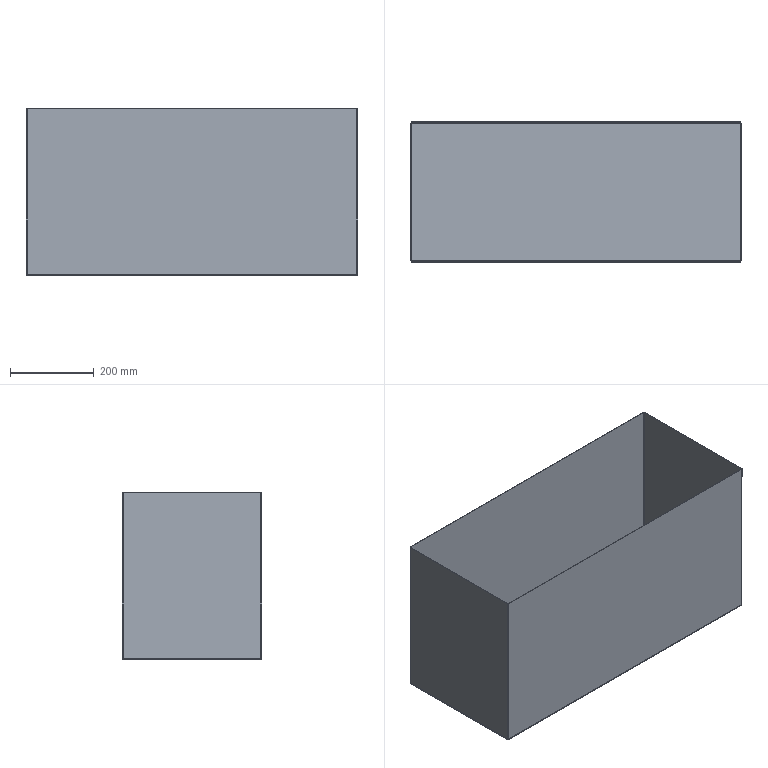Part | SolidWorks | features EdgeFlange 1, FlatPattern 1, SMBaseFlange 1, SheetMetal 1 | 1 solid | 38 faces | box 795 x 335 x 400 mm | volume 2310463 mm3 | plane 22 | spline 8 | cylinder 8 | commonest cylinder face diameters 2 x4 6 x4
STEP:
#1=CARTESIAN_POINT('',(-394.5,-164.5,-2.));
#2=VERTEX_POINT('',#1);
#3=CARTESIAN_POINT('',(-394.5,164.5,-2.));
#4=VERTEX_POINT('',#3);
#5=CARTESIAN_POINT('',(-394.5,-164.793,-2.));
#6=DIRECTION('',(0.,1.,0.));
#7=VECTOR('',#6,1000.);
#8=LINE('',#5,#7);
#9=EDGE_CURVE('',#2,#4,#8,.T.);
#10=ORIENTED_EDGE('',*,*,#9,.T.);
#11=CARTESIAN_POINT('',(394.5,164.5,-2.));
#12=VERTEX_POINT('',#11);
#13=CARTESIAN_POINT('',(-394.793,164.5,-2.));
#14=DIRECTION('',(1.,0.,0.));
#15=VECTOR('',#14,1000.);
#16=LINE('',#13,#15);
#17=EDGE_CURVE('',#4,#12,#16,.T.);
#18=ORIENTED_EDGE('',*,*,#17,.T.);
#19=CARTESIAN_POINT('',(394.5,-164.5,-2.));
#20=VERTEX_POINT('',#19);
#21=CARTESIAN_POINT('',(394.5,164.793,-2.));
#22=DIRECTION('',(0.,-1.,0.));
#23=VECTOR('',#22,1000.);
#24=LINE('',#21,#23);
#25=EDGE_CURVE('',#12,#20,#24,.T.);
#26=ORIENTED_EDGE('',*,*,#25,.T.);
#27=CARTESIAN_POINT('',(394.793,-164.5,-2.));
#28=DIRECTION('',(-1.,0.,0.));
#29=VECTOR('',#28,1000.);
#30=LINE('',#27,#29);
#31=EDGE_CURVE('',#20,#2,#30,.T.);
#32=ORIENTED_EDGE('',*,*,#31,.T.);
#33=EDGE_LOOP('',(#10,#18,#26,#32));
#34=FACE_OUTER_BOUND('',#33,.T.);
#35=CARTESIAN_POINT('',(0.,0.,-2.));
#36=DIRECTION('',(0.,0.,1.));
#37=DIRECTION('',(1.,0.,0.));
#38=AXIS2_PLACEMENT_3D('',#35,#36,#37);
#39=PLANE('',#38);
#40=ADVANCED_FACE('',(#34),#39,.F.);
#41=CARTESIAN_POINT('',(-394.5,164.5,0.));
#42=VERTEX_POINT('',#41);
#43=CARTESIAN_POINT('',(394.5,164.5,0.));
#44=VERTEX_POINT('',#43);
#45=CARTESIAN_POINT('',(-394.793,164.5,0.));
#46=DIRECTION('',(1.,0.,0.));
#47=VECTOR('',#46,1000.);
#48=LINE('',#45,#47);
#49=EDGE_CURVE('',#42,#44,#48,.T.);
#50=ORIENTED_EDGE('',*,*,#49,.F.);
#51=CARTESIAN_POINT('',(-394.5,-164.5,0.));
#52=VERTEX_POINT('',#51);
#53=CARTESIAN_POINT('',(-394.5,-164.793,0.));
#54=DIRECTION('',(0.,1.,0.));
#55=VECTOR('',#54,1000.);
#56=LINE('',#53,#55);
#57=EDGE_CURVE('',#52,#42,#56,.T.);
#58=ORIENTED_EDGE('',*,*,#57,.F.);
#59=CARTESIAN_POINT('',(394.5,-164.5,0.));
#60=VERTEX_POINT('',#59);
#61=CARTESIAN_POINT('',(394.793,-164.5,0.));
#62=DIRECTION('',(-1.,0.,0.));
#63=VECTOR('',#62,1000.);
#64=LINE('',#61,#63);
#65=EDGE_CURVE('',#60,#52,#64,.T.);
#66=ORIENTED_EDGE('',*,*,#65,.F.);
#67=CARTESIAN_POINT('',(394.5,164.793,0.));
#68=DIRECTION('',(0.,-1.,0.));
#69=VECTOR('',#68,1000.);
#70=LINE('',#67,#69);
#71=EDGE_CURVE('',#44,#60,#70,.T.);
#72=ORIENTED_EDGE('',*,*,#71,.F.);
#73=EDGE_LOOP('',(#50,#58,#66,#72));
#74=FACE_OUTER_BOUND('',#73,.T.);
#75=CARTESIAN_POINT('',(0.,0.,0.));
#76=DIRECTION('',(0.,0.,1.));
#77=DIRECTION('',(1.,0.,0.));
#78=AXIS2_PLACEMENT_3D('',#75,#76,#77);
#79=PLANE('',#78);
#80=ADVANCED_FACE('',(#74),#79,.T.);
#81=CARTESIAN_POINT('',(394.793,167.5,1.));
#82=VERTEX_POINT('',#81);
#83=CARTESIAN_POINT('',(394.793,165.5,1.));
#84=VERTEX_POINT('',#83);
#85=CARTESIAN_POINT('',(394.793,165.5,1.));
#86=DIRECTION('',(0.,-1.,0.));
#87=VECTOR('',#86,1000.);
#88=LINE('',#85,#87);
#89=EDGE_CURVE('',#82,#84,#88,.T.);
#90=ORIENTED_EDGE('',*,*,#89,.T.);
#91=CARTESIAN_POINT('',(394.5,164.5,0.));
#92=CARTESIAN_POINT('',(394.549,164.762,0.));
#93=CARTESIAN_POINT('',(394.598,165.022,0.1078));
#94=CARTESIAN_POINT('',(394.695,165.392,0.478));
#95=CARTESIAN_POINT('',(394.744,165.5,0.7382));
#96=CARTESIAN_POINT('',(394.793,165.5,1.));
#97=B_SPLINE_CURVE_WITH_KNOTS('',3,(#91,#92,#93,#94,#95,#96),.UNSPECIFIED.,.F.,.F.,(4,2,4),(0.,0.5,1.),.UNSPECIFIED.);
#98=EDGE_CURVE('',#44,#84,#97,.T.);
#99=ORIENTED_EDGE('',*,*,#98,.F.);
#100=CARTESIAN_POINT('',(394.5,164.5,0.));
#101=DIRECTION('',(0.,0.,-1.));
#102=VECTOR('',#101,1000.);
#103=LINE('',#100,#102);
#104=EDGE_CURVE('',#44,#12,#103,.T.);
#105=ORIENTED_EDGE('',*,*,#104,.T.);
#106=CARTESIAN_POINT('',(394.5,164.5,-2.));
#107=CARTESIAN_POINT('',(394.524,164.893,-2.));
#108=CARTESIAN_POINT('',(394.549,165.285,-1.922));
#109=CARTESIAN_POINT('',(394.598,166.011,-1.621));
#110=CARTESIAN_POINT('',(394.622,166.344,-1.399));
#111=CARTESIAN_POINT('',(394.671,166.899,-0.8436));
#112=CARTESIAN_POINT('',(394.695,167.121,-0.5109));
#113=CARTESIAN_POINT('',(394.744,167.422,0.2148));
#114=CARTESIAN_POINT('',(394.768,167.5,0.6073));
#115=CARTESIAN_POINT('',(394.793,167.5,1.));
#116=B_SPLINE_CURVE_WITH_KNOTS('',3,(#106,#107,#108,#109,#110,#111,#112,#113,#114,#115),.UNSPECIFIED.,.F.,.F.,(4,2,2,2,4),(0.,0.25,0.5,0.75,1.),.UNSPECIFIED.);
#117=EDGE_CURVE('',#12,#82,#116,.T.);
#118=ORIENTED_EDGE('',*,*,#117,.T.);
#119=EDGE_LOOP('',(#90,#99,#105,#118));
#120=FACE_OUTER_BOUND('',#119,.T.);
#121=CARTESIAN_POINT('',(394.5,164.5,-2.02));
#122=CARTESIAN_POINT('',(394.524,164.895,-2.02));
#123=CARTESIAN_POINT('',(394.549,165.29,-1.941));
#124=CARTESIAN_POINT('',(394.598,166.021,-1.639));
#125=CARTESIAN_POINT('',(394.622,166.356,-1.415));
#126=CARTESIAN_POINT('',(394.671,166.915,-0.8559));
#127=CARTESIAN_POINT('',(394.695,167.139,-0.5209));
#128=CARTESIAN_POINT('',(394.744,167.441,0.2095));
#129=CARTESIAN_POINT('',(394.768,167.52,0.6046));
#130=CARTESIAN_POINT('',(394.793,167.52,1.));
#131=CARTESIAN_POINT('',(394.5,164.5,-2.));
#132=CARTESIAN_POINT('',(394.524,164.893,-2.));
#133=CARTESIAN_POINT('',(394.549,165.285,-1.922));
#134=CARTESIAN_POINT('',(394.598,166.011,-1.621));
#135=CARTESIAN_POINT('',(394.622,166.344,-1.399));
#136=CARTESIAN_POINT('',(394.671,166.899,-0.8436));
#137=CARTESIAN_POINT('',(394.695,167.121,-0.5109));
#138=CARTESIAN_POINT('',(394.744,167.422,0.2148));
#139=CARTESIAN_POINT('',(394.768,167.5,0.6072));
#140=CARTESIAN_POINT('',(394.793,167.5,1.));
#141=CARTESIAN_POINT('',(394.5,164.5,0.));
#142=CARTESIAN_POINT('',(394.524,164.631,0.));
#143=CARTESIAN_POINT('',(394.549,164.762,0.02603));
#144=CARTESIAN_POINT('',(394.598,165.004,0.1262));
#145=CARTESIAN_POINT('',(394.622,165.115,0.2003));
#146=CARTESIAN_POINT('',(394.671,165.3,0.3855));
#147=CARTESIAN_POINT('',(394.695,165.374,0.4964));
#148=CARTESIAN_POINT('',(394.744,165.474,0.7383));
#149=CARTESIAN_POINT('',(394.768,165.5,0.8691));
#150=CARTESIAN_POINT('',(394.793,165.5,1.));
#151=CARTESIAN_POINT('',(394.5,164.5,0.0202));
#152=CARTESIAN_POINT('',(394.524,164.628,0.0202));
#153=CARTESIAN_POINT('',(394.549,164.756,0.0457));
#154=CARTESIAN_POINT('',(394.598,164.993,0.1439));
#155=CARTESIAN_POINT('',(394.622,165.102,0.2165));
#156=CARTESIAN_POINT('',(394.671,165.284,0.3979));
#157=CARTESIAN_POINT('',(394.695,165.356,0.5066));
#158=CARTESIAN_POINT('',(394.744,165.454,0.7435));
#159=CARTESIAN_POINT('',(394.768,165.48,0.8717));
#160=CARTESIAN_POINT('',(394.793,165.48,1.));
#161=B_SPLINE_SURFACE_WITH_KNOTS('',1,3,((#121,#122,#123,#124,#125,#126,#127,#128,#129,#130),(#131,#132,#133,#134,#135,#136,#137,#138,#139,#140),(#141,#142,#143,#144,#145,#146,#147,#148,#149,#150),(#151,#152,#153,#154,#155,#156,#157,#158,#159,#160)),.UNSPECIFIED.,.F.,.F.,.F.,(2,1,1,2),(4,2,2,2,4),(-0.01,0.,1.,1.01),(0.,0.25,0.5,0.75,1.),.UNSPECIFIED.);
#162=ADVANCED_FACE('',(#120),#161,.F.);
#163=CARTESIAN_POINT('',(-394.793,165.5,1.));
#164=VERTEX_POINT('',#163);
#165=CARTESIAN_POINT('',(-394.793,165.5,1.));
#166=CARTESIAN_POINT('',(-394.744,165.5,0.7382));
#167=CARTESIAN_POINT('',(-394.695,165.392,0.478));
#168=CARTESIAN_POINT('',(-394.598,165.022,0.1078));
#169=CARTESIAN_POINT('',(-394.549,164.762,0.));
#170=CARTESIAN_POINT('',(-394.5,164.5,0.));
#171=B_SPLINE_CURVE_WITH_KNOTS('',3,(#165,#166,#167,#168,#169,#170),.UNSPECIFIED.,.F.,.F.,(4,2,4),(0.,0.5,1.),.UNSPECIFIED.);
#172=EDGE_CURVE('',#164,#42,#171,.T.);
#173=ORIENTED_EDGE('',*,*,#172,.F.);
#174=CARTESIAN_POINT('',(-394.793,167.5,1.));
#175=VERTEX_POINT('',#174);
#176=CARTESIAN_POINT('',(-394.793,165.5,1.));
#177=DIRECTION('',(0.,-1.,0.));
#178=VECTOR('',#177,1000.);
#179=LINE('',#176,#178);
#180=EDGE_CURVE('',#175,#164,#179,.T.);
#181=ORIENTED_EDGE('',*,*,#180,.F.);
#182=CARTESIAN_POINT('',(-394.793,167.5,1.));
#183=CARTESIAN_POINT('',(-394.768,167.5,0.6073));
#184=CARTESIAN_POINT('',(-394.744,167.422,0.2148));
#185=CARTESIAN_POINT('',(-394.695,167.121,-0.5109));
#186=CARTESIAN_POINT('',(-394.671,166.899,-0.8436));
#187=CARTESIAN_POINT('',(-394.622,166.344,-1.399));
#188=CARTESIAN_POINT('',(-394.598,166.011,-1.621));
#189=CARTESIAN_POINT('',(-394.549,165.285,-1.922));
#190=CARTESIAN_POINT('',(-394.524,164.893,-2.));
#191=CARTESIAN_POINT('',(-394.5,164.5,-2.));
#192=B_SPLINE_CURVE_WITH_KNOTS('',3,(#182,#183,#184,#185,#186,#187,#188,#189,#190,#191),.UNSPECIFIED.,.F.,.F.,(4,2,2,2,4),(0.,0.25,0.5,0.75,1.),.UNSPECIFIED.);
#193=EDGE_CURVE('',#175,#4,#192,.T.);
#194=ORIENTED_EDGE('',*,*,#193,.T.);
#195=CARTESIAN_POINT('',(-394.5,164.5,0.));
#196=DIRECTION('',(0.,0.,-1.));
#197=VECTOR('',#196,1000.);
#198=LINE('',#195,#197);
#199=EDGE_CURVE('',#42,#4,#198,.T.);
#200=ORIENTED_EDGE('',*,*,#199,.F.);
#201=EDGE_LOOP('',(#173,#181,#194,#200));
#202=FACE_OUTER_BOUND('',#201,.T.);
#203=CARTESIAN_POINT('',(-394.793,167.52,1.));
#204=CARTESIAN_POINT('',(-394.768,167.52,0.6046));
#205=CARTESIAN_POINT('',(-394.744,167.441,0.2095));
#206=CARTESIAN_POINT('',(-394.695,167.139,-0.5209));
#207=CARTESIAN_POINT('',(-394.671,166.915,-0.8559));
#208=CARTESIAN_POINT('',(-394.622,166.356,-1.415));
#209=CARTESIAN_POINT('',(-394.598,166.021,-1.639));
#210=CARTESIAN_POINT('',(-394.549,165.29,-1.941));
#211=CARTESIAN_POINT('',(-394.524,164.895,-2.02));
#212=CARTESIAN_POINT('',(-394.5,164.5,-2.02));
#213=CARTESIAN_POINT('',(-394.793,167.5,1.));
#214=CARTESIAN_POINT('',(-394.768,167.5,0.6072));
#215=CARTESIAN_POINT('',(-394.744,167.422,0.2148));
#216=CARTESIAN_POINT('',(-394.695,167.121,-0.5109));
#217=CARTESIAN_POINT('',(-394.671,166.899,-0.8436));
#218=CARTESIAN_POINT('',(-394.622,166.344,-1.399));
#219=CARTESIAN_POINT('',(-394.598,166.011,-1.621));
#220=CARTESIAN_POINT('',(-394.549,165.285,-1.922));
#221=CARTESIAN_POINT('',(-394.524,164.893,-2.));
#222=CARTESIAN_POINT('',(-394.5,164.5,-2.));
#223=CARTESIAN_POINT('',(-394.793,165.5,1.));
#224=CARTESIAN_POINT('',(-394.768,165.5,0.8691));
#225=CARTESIAN_POINT('',(-394.744,165.474,0.7383));
#226=CARTESIAN_POINT('',(-394.695,165.374,0.4964));
#227=CARTESIAN_POINT('',(-394.671,165.3,0.3855));
#228=CARTESIAN_POINT('',(-394.622,165.115,0.2003));
#229=CARTESIAN_POINT('',(-394.598,165.004,0.1262));
#230=CARTESIAN_POINT('',(-394.549,164.762,0.02603));
#231=CARTESIAN_POINT('',(-394.524,164.631,0.));
#232=CARTESIAN_POINT('',(-394.5,164.5,0.));
#233=CARTESIAN_POINT('',(-394.793,165.48,1.));
#234=CARTESIAN_POINT('',(-394.768,165.48,0.8717));
#235=CARTESIAN_POINT('',(-394.744,165.454,0.7435));
#236=CARTESIAN_POINT('',(-394.695,165.356,0.5066));
#237=CARTESIAN_POINT('',(-394.671,165.284,0.3979));
#238=CARTESIAN_POINT('',(-394.622,165.102,0.2165));
#239=CARTESIAN_POINT('',(-394.598,164.993,0.1439));
#240=CARTESIAN_POINT('',(-394.549,164.756,0.0457));
#241=CARTESIAN_POINT('',(-394.524,164.628,0.0202));
#242=CARTESIAN_POINT('',(-394.5,164.5,0.0202));
#243=B_SPLINE_SURFACE_WITH_KNOTS('',1,3,((#203,#204,#205,#206,#207,#208,#209,#210,#211,#212),(#213,#214,#215,#216,#217,#218,#219,#220,#221,#222),(#223,#224,#225,#226,#227,#228,#229,#230,#231,#232),(#233,#234,#235,#236,#237,#238,#239,#240,#241,#242)),.UNSPECIFIED.,.F.,.F.,.F.,(2,1,1,2),(4,2,2,2,4),(-0.01,0.,1.,1.01),(0.,0.25,0.5,0.75,1.),.UNSPECIFIED.);
#244=ADVANCED_FACE('',(#202),#243,.F.);
#245=ORIENTED_EDGE('',*,*,#17,.F.);
#246=ORIENTED_EDGE('',*,*,#193,.F.);
#247=CARTESIAN_POINT('',(397.5,167.5,1.));
#248=DIRECTION('',(1.,0.,0.));
#249=VECTOR('',#248,1000.);
#250=LINE('',#247,#249);
#251=EDGE_CURVE('',#175,#82,#250,.T.);
#252=ORIENTED_EDGE('',*,*,#251,.T.);
#253=ORIENTED_EDGE('',*,*,#117,.F.);
#254=EDGE_LOOP('',(#245,#246,#252,#253));
#255=FACE_OUTER_BOUND('',#254,.T.);
#256=CARTESIAN_POINT('',(-394.793,164.5,1.));
#257=DIRECTION('',(-1.,0.,0.));
#258=DIRECTION('',(0.,1.,0.));
#259=AXIS2_PLACEMENT_3D('',#256,#257,#258);
#260=CYLINDRICAL_SURFACE('',#259,3.);
#261=ADVANCED_FACE('',(#255),#260,.T.);
#262=ORIENTED_EDGE('',*,*,#49,.T.);
#263=ORIENTED_EDGE('',*,*,#98,.T.);
#264=CARTESIAN_POINT('',(397.5,165.5,1.));
#265=DIRECTION('',(-1.,0.,0.));
#266=VECTOR('',#265,1000.);
#267=LINE('',#264,#266);
#268=EDGE_CURVE('',#84,#164,#267,.T.);
#269=ORIENTED_EDGE('',*,*,#268,.T.);
#270=ORIENTED_EDGE('',*,*,#172,.T.);
#271=EDGE_LOOP('',(#262,#263,#269,#270));
#272=FACE_OUTER_BOUND('',#271,.T.);
#273=CARTESIAN_POINT('',(-394.793,164.5,1.));
#274=DIRECTION('',(-1.,0.,0.));
#275=DIRECTION('',(0.,1.,0.));
#276=AXIS2_PLACEMENT_3D('',#273,#274,#275);
#277=CYLINDRICAL_SURFACE('',#276,1.);
#278=ADVANCED_FACE('',(#272),#277,.F.);
#279=CARTESIAN_POINT('',(394.793,167.5,398.));
#280=VERTEX_POINT('',#279);
#281=CARTESIAN_POINT('',(394.793,167.5,0.));
#282=DIRECTION('',(0.,0.,1.));
#283=VECTOR('',#282,1000.);
#284=LINE('',#281,#283);
#285=EDGE_CURVE('',#82,#280,#284,.T.);
#286=ORIENTED_EDGE('',*,*,#285,.T.);
#287=CARTESIAN_POINT('',(394.793,165.5,398.));
#288=VERTEX_POINT('',#287);
#289=CARTESIAN_POINT('',(394.793,165.5,398.));
#290=DIRECTION('',(0.,-1.,0.));
#291=VECTOR('',#290,1000.);
#292=LINE('',#289,#291);
#293=EDGE_CURVE('',#280,#288,#292,.T.);
#294=ORIENTED_EDGE('',*,*,#293,.T.);
#295=CARTESIAN_POINT('',(394.793,165.5,0.));
#296=DIRECTION('',(0.,0.,1.));
#297=VECTOR('',#296,1000.);
#298=LINE('',#295,#297);
#299=EDGE_CURVE('',#84,#288,#298,.T.);
#300=ORIENTED_EDGE('',*,*,#299,.F.);
#301=ORIENTED_EDGE('',*,*,#89,.F.);
#302=EDGE_LOOP('',(#286,#294,#300,#301));
#303=FACE_OUTER_BOUND('',#302,.T.);
#304=CARTESIAN_POINT('',(394.793,165.5,0.));
#305=DIRECTION('',(1.,0.,0.));
#306=DIRECTION('',(0.,0.,-1.));
#307=AXIS2_PLACEMENT_3D('',#304,#305,#306);
#308=PLANE('',#307);
#309=ADVANCED_FACE('',(#303),#308,.T.);
#310=ORIENTED_EDGE('',*,*,#251,.F.);
#311=CARTESIAN_POINT('',(-394.793,167.5,398.));
#312=VERTEX_POINT('',#311);
#313=CARTESIAN_POINT('',(-394.793,167.5,0.));
#314=DIRECTION('',(0.,0.,1.));
#315=VECTOR('',#314,1000.);
#316=LINE('',#313,#315);
#317=EDGE_CURVE('',#175,#312,#316,.T.);
#318=ORIENTED_EDGE('',*,*,#317,.T.);
#319=CARTESIAN_POINT('',(0.,167.5,398.));
#320=DIRECTION('',(1.,0.,0.));
#321=VECTOR('',#320,1000.);
#322=LINE('',#319,#321);
#323=EDGE_CURVE('',#312,#280,#322,.T.);
#324=ORIENTED_EDGE('',*,*,#323,.T.);
#325=ORIENTED_EDGE('',*,*,#285,.F.);
#326=EDGE_LOOP('',(#310,#318,#324,#325));
#327=FACE_OUTER_BOUND('',#326,.T.);
#328=CARTESIAN_POINT('',(0.,167.5,0.));
#329=DIRECTION('',(0.,-1.,0.));
#330=DIRECTION('',(0.,0.,-1.));
#331=AXIS2_PLACEMENT_3D('',#328,#329,#330);
#332=PLANE('',#331);
#333=ADVANCED_FACE('',(#327),#332,.F.);
#334=CARTESIAN_POINT('',(-394.793,165.5,398.));
#335=VERTEX_POINT('',#334);
#336=CARTESIAN_POINT('',(-394.793,165.5,0.));
#337=DIRECTION('',(0.,0.,1.));
#338=VECTOR('',#337,1000.);
#339=LINE('',#336,#338);
#340=EDGE_CURVE('',#164,#335,#339,.T.);
#341=ORIENTED_EDGE('',*,*,#340,.F.);
#342=ORIENTED_EDGE('',*,*,#268,.F.);
#343=ORIENTED_EDGE('',*,*,#299,.T.);
#344=CARTESIAN_POINT('',(397.5,165.5,398.));
#345=DIRECTION('',(1.,0.,0.));
#346=VECTOR('',#345,1000.);
#347=LINE('',#344,#346);
#348=EDGE_CURVE('',#335,#288,#347,.T.);
#349=ORIENTED_EDGE('',*,*,#348,.F.);
#350=EDGE_LOOP('',(#341,#342,#343,#349));
#351=FACE_OUTER_BOUND('',#350,.T.);
#352=CARTESIAN_POINT('',(0.,165.5,0.));
#353=DIRECTION('',(0.,-1.,0.));
#354=DIRECTION('',(0.,0.,-1.));
#355=AXIS2_PLACEMENT_3D('',#352,#353,#354);
#356=PLANE('',#355);
#357=ADVANCED_FACE('',(#351),#356,.T.);
#358=ORIENTED_EDGE('',*,*,#323,.F.);
#359=CARTESIAN_POINT('',(-394.793,167.5,398.));
#360=DIRECTION('',(0.,-1.,0.));
#361=VECTOR('',#360,1000.);
#362=LINE('',#359,#361);
#363=EDGE_CURVE('',#312,#335,#362,.T.);
#364=ORIENTED_EDGE('',*,*,#363,.T.);
#365=ORIENTED_EDGE('',*,*,#348,.T.);
#366=ORIENTED_EDGE('',*,*,#293,.F.);
#367=EDGE_LOOP('',(#358,#364,#365,#366));
#368=FACE_OUTER_BOUND('',#367,.T.);
#369=CARTESIAN_POINT('',(397.5,167.5,398.));
#370=DIRECTION('',(0.,0.,-1.));
#371=DIRECTION('',(0.,1.,0.));
#372=AXIS2_PLACEMENT_3D('',#369,#370,#371);
#373=PLANE('',#372);
#374=ADVANCED_FACE('',(#368),#373,.F.);
#375=ORIENTED_EDGE('',*,*,#363,.F.);
#376=ORIENTED_EDGE('',*,*,#317,.F.);
#377=ORIENTED_EDGE('',*,*,#180,.T.);
#378=ORIENTED_EDGE('',*,*,#340,.T.);
#379=EDGE_LOOP('',(#375,#376,#377,#378));
#380=FACE_OUTER_BOUND('',#379,.T.);
#381=CARTESIAN_POINT('',(-394.793,165.5,0.));
#382=DIRECTION('',(1.,0.,0.));
#383=DIRECTION('',(0.,0.,-1.));
#384=AXIS2_PLACEMENT_3D('',#381,#382,#383);
#385=PLANE('',#384);
#386=ADVANCED_FACE('',(#380),#385,.F.);
#387=CARTESIAN_POINT('',(-394.793,-167.5,1.));
#388=VERTEX_POINT('',#387);
#389=CARTESIAN_POINT('',(-394.793,-165.5,1.));
#390=VERTEX_POINT('',#389);
#391=CARTESIAN_POINT('',(-394.793,-165.5,1.));
#392=DIRECTION('',(0.,1.,0.));
#393=VECTOR('',#392,1000.);
#394=LINE('',#391,#393);
#395=EDGE_CURVE('',#388,#390,#394,.T.);
#396=ORIENTED_EDGE('',*,*,#395,.T.);
#397=CARTESIAN_POINT('',(-394.5,-164.5,0.));
#398=CARTESIAN_POINT('',(-394.549,-164.762,0.));
#399=CARTESIAN_POINT('',(-394.598,-165.022,0.1078));
#400=CARTESIAN_POINT('',(-394.695,-165.392,0.478));
#401=CARTESIAN_POINT('',(-394.744,-165.5,0.7382));
#402=CARTESIAN_POINT('',(-394.793,-165.5,1.));
#403=B_SPLINE_CURVE_WITH_KNOTS('',3,(#397,#398,#399,#400,#401,#402),.UNSPECIFIED.,.F.,.F.,(4,2,4),(0.,0.5,1.),.UNSPECIFIED.);
#404=EDGE_CURVE('',#52,#390,#403,.T.);
#405=ORIENTED_EDGE('',*,*,#404,.F.);
#406=CARTESIAN_POINT('',(-394.5,-164.5,0.));
#407=DIRECTION('',(0.,0.,-1.));
#408=VECTOR('',#407,1000.);
#409=LINE('',#406,#408);
#410=EDGE_CURVE('',#52,#2,#409,.T.);
#411=ORIENTED_EDGE('',*,*,#410,.T.);
#412=CARTESIAN_POINT('',(-394.5,-164.5,-2.));
#413=CARTESIAN_POINT('',(-394.524,-164.893,-2.));
#414=CARTESIAN_POINT('',(-394.549,-165.285,-1.922));
#415=CARTESIAN_POINT('',(-394.598,-166.011,-1.621));
#416=CARTESIAN_POINT('',(-394.622,-166.344,-1.399));
#417=CARTESIAN_POINT('',(-394.671,-166.899,-0.8436));
#418=CARTESIAN_POINT('',(-394.695,-167.121,-0.5109));
#419=CARTESIAN_POINT('',(-394.744,-167.422,0.2148));
#420=CARTESIAN_POINT('',(-394.768,-167.5,0.6073));
#421=CARTESIAN_POINT('',(-394.793,-167.5,1.));
#422=B_SPLINE_CURVE_WITH_KNOTS('',3,(#412,#413,#414,#415,#416,#417,#418,#419,#420,#421),.UNSPECIFIED.,.F.,.F.,(4,2,2,2,4),(0.,0.25,0.5,0.75,1.),.UNSPECIFIED.);
#423=EDGE_CURVE('',#2,#388,#422,.T.);
#424=ORIENTED_EDGE('',*,*,#423,.T.);
#425=EDGE_LOOP('',(#396,#405,#411,#424));
#426=FACE_OUTER_BOUND('',#425,.T.);
#427=CARTESIAN_POINT('',(-394.5,-164.5,-2.02));
#428=CARTESIAN_POINT('',(-394.524,-164.895,-2.02));
#429=CARTESIAN_POINT('',(-394.549,-165.29,-1.941));
#430=CARTESIAN_POINT('',(-394.598,-166.021,-1.639));
#431=CARTESIAN_POINT('',(-394.622,-166.356,-1.415));
#432=CARTESIAN_POINT('',(-394.671,-166.915,-0.8559));
#433=CARTESIAN_POINT('',(-394.695,-167.139,-0.5209));
#434=CARTESIAN_POINT('',(-394.744,-167.441,0.2095));
#435=CARTESIAN_POINT('',(-394.768,-167.52,0.6046));
#436=CARTESIAN_POINT('',(-394.793,-167.52,1.));
#437=CARTESIAN_POINT('',(-394.5,-164.5,-2.));
#438=CARTESIAN_POINT('',(-394.524,-164.893,-2.));
#439=CARTESIAN_POINT('',(-394.549,-165.285,-1.922));
#440=CARTESIAN_POINT('',(-394.598,-166.011,-1.621));
#441=CARTESIAN_POINT('',(-394.622,-166.344,-1.399));
#442=CARTESIAN_POINT('',(-394.671,-166.899,-0.8436));
#443=CARTESIAN_POINT('',(-394.695,-167.121,-0.5109));
#444=CARTESIAN_POINT('',(-394.744,-167.422,0.2148));
#445=CARTESIAN_POINT('',(-394.768,-167.5,0.6072));
#446=CARTESIAN_POINT('',(-394.793,-167.5,1.));
#447=CARTESIAN_POINT('',(-394.5,-164.5,0.));
#448=CARTESIAN_POINT('',(-394.524,-164.631,0.));
#449=CARTESIAN_POINT('',(-394.549,-164.762,0.02603));
#450=CARTESIAN_POINT('',(-394.598,-165.004,0.1262));
#451=CARTESIAN_POINT('',(-394.622,-165.115,0.2003));
#452=CARTESIAN_POINT('',(-394.671,-165.3,0.3855));
#453=CARTESIAN_POINT('',(-394.695,-165.374,0.4964));
#454=CARTESIAN_POINT('',(-394.744,-165.474,0.7383));
#455=CARTESIAN_POINT('',(-394.768,-165.5,0.8691));
#456=CARTESIAN_POINT('',(-394.793,-165.5,1.));
#457=CARTESIAN_POINT('',(-394.5,-164.5,0.0202));
#458=CARTESIAN_POINT('',(-394.524,-164.628,0.0202));
#459=CARTESIAN_POINT('',(-394.549,-164.756,0.0457));
#460=CARTESIAN_POINT('',(-394.598,-164.993,0.1439));
#461=CARTESIAN_POINT('',(-394.622,-165.102,0.2165));
#462=CARTESIAN_POINT('',(-394.671,-165.284,0.3979));
#463=CARTESIAN_POINT('',(-394.695,-165.356,0.5066));
#464=CARTESIAN_POINT('',(-394.744,-165.454,0.7435));
#465=CARTESIAN_POINT('',(-394.768,-165.48,0.8717));
#466=CARTESIAN_POINT('',(-394.793,-165.48,1.));
#467=B_SPLINE_SURFACE_WITH_KNOTS('',1,3,((#427,#428,#429,#430,#431,#432,#433,#434,#435,#436),(#437,#438,#439,#440,#441,#442,#443,#444,#445,#446),(#447,#448,#449,#450,#451,#452,#453,#454,#455,#456),(#457,#458,#459,#460,#461,#462,#463,#464,#465,#466)),.UNSPECIFIED.,.F.,.F.,.F.,(2,1,1,2),(4,2,2,2,4),(-0.01,0.,1.,1.01),(0.,0.25,0.5,0.75,1.),.UNSPECIFIED.);
#468=ADVANCED_FACE('',(#426),#467,.F.);
#469=CARTESIAN_POINT('',(394.793,-165.5,1.));
#470=VERTEX_POINT('',#469);
#471=CARTESIAN_POINT('',(394.793,-165.5,1.));
#472=CARTESIAN_POINT('',(394.744,-165.5,0.7382));
#473=CARTESIAN_POINT('',(394.695,-165.392,0.478));
#474=CARTESIAN_POINT('',(394.598,-165.022,0.1078));
#475=CARTESIAN_POINT('',(394.549,-164.762,0.));
#476=CARTESIAN_POINT('',(394.5,-164.5,0.));
#477=B_SPLINE_CURVE_WITH_KNOTS('',3,(#471,#472,#473,#474,#475,#476),.UNSPECIFIED.,.F.,.F.,(4,2,4),(0.,0.5,1.),.UNSPECIFIED.);
#478=EDGE_CURVE('',#470,#60,#477,.T.);
#479=ORIENTED_EDGE('',*,*,#478,.F.);
#480=CARTESIAN_POINT('',(394.793,-167.5,1.));
#481=VERTEX_POINT('',#480);
#482=CARTESIAN_POINT('',(394.793,-165.5,1.));
#483=DIRECTION('',(0.,1.,0.));
#484=VECTOR('',#483,1000.);
#485=LINE('',#482,#484);
#486=EDGE_CURVE('',#481,#470,#485,.T.);
#487=ORIENTED_EDGE('',*,*,#486,.F.);
#488=CARTESIAN_POINT('',(394.793,-167.5,1.));
#489=CARTESIAN_POINT('',(394.768,-167.5,0.6073));
#490=CARTESIAN_POINT('',(394.744,-167.422,0.2148));
#491=CARTESIAN_POINT('',(394.695,-167.121,-0.5109));
#492=CARTESIAN_POINT('',(394.671,-166.899,-0.8436));
#493=CARTESIAN_POINT('',(394.622,-166.344,-1.399));
#494=CARTESIAN_POINT('',(394.598,-166.011,-1.621));
#495=CARTESIAN_POINT('',(394.549,-165.285,-1.922));
#496=CARTESIAN_POINT('',(394.524,-164.893,-2.));
#497=CARTESIAN_POINT('',(394.5,-164.5,-2.));
#498=B_SPLINE_CURVE_WITH_KNOTS('',3,(#488,#489,#490,#491,#492,#493,#494,#495,#496,#497),.UNSPECIFIED.,.F.,.F.,(4,2,2,2,4),(0.,0.25,0.5,0.75,1.),.UNSPECIFIED.);
#499=EDGE_CURVE('',#481,#20,#498,.T.);
#500=ORIENTED_EDGE('',*,*,#499,.T.);
#501=CARTESIAN_POINT('',(394.5,-164.5,0.));
#502=DIRECTION('',(0.,0.,-1.));
#503=VECTOR('',#502,1000.);
#504=LINE('',#501,#503);
#505=EDGE_CURVE('',#60,#20,#504,.T.);
#506=ORIENTED_EDGE('',*,*,#505,.F.);
#507=EDGE_LOOP('',(#479,#487,#500,#506));
#508=FACE_OUTER_BOUND('',#507,.T.);
#509=CARTESIAN_POINT('',(394.793,-167.52,1.));
#510=CARTESIAN_POINT('',(394.768,-167.52,0.6046));
#511=CARTESIAN_POINT('',(394.744,-167.441,0.2095));
#512=CARTESIAN_POINT('',(394.695,-167.139,-0.5209));
#513=CARTESIAN_POINT('',(394.671,-166.915,-0.8559));
#514=CARTESIAN_POINT('',(394.622,-166.356,-1.415));
#515=CARTESIAN_POINT('',(394.598,-166.021,-1.639));
#516=CARTESIAN_POINT('',(394.549,-165.29,-1.941));
#517=CARTESIAN_POINT('',(394.524,-164.895,-2.02));
#518=CARTESIAN_POINT('',(394.5,-164.5,-2.02));
#519=CARTESIAN_POINT('',(394.793,-167.5,1.));
#520=CARTESIAN_POINT('',(394.768,-167.5,0.6072));
#521=CARTESIAN_POINT('',(394.744,-167.422,0.2148));
#522=CARTESIAN_POINT('',(394.695,-167.121,-0.5109));
#523=CARTESIAN_POINT('',(394.671,-166.899,-0.8436));
#524=CARTESIAN_POINT('',(394.622,-166.344,-1.399));
#525=CARTESIAN_POINT('',(394.598,-166.011,-1.621));
#526=CARTESIAN_POINT('',(394.549,-165.285,-1.922));
#527=CARTESIAN_POINT('',(394.524,-164.893,-2.));
#528=CARTESIAN_POINT('',(394.5,-164.5,-2.));
#529=CARTESIAN_POINT('',(394.793,-165.5,1.));
#530=CARTESIAN_POINT('',(394.768,-165.5,0.8691));
#531=CARTESIAN_POINT('',(394.744,-165.474,0.7383));
#532=CARTESIAN_POINT('',(394.695,-165.374,0.4964));
#533=CARTESIAN_POINT('',(394.671,-165.3,0.3855));
#534=CARTESIAN_POINT('',(394.622,-165.115,0.2003));
#535=CARTESIAN_POINT('',(394.598,-165.004,0.1262));
#536=CARTESIAN_POINT('',(394.549,-164.762,0.02603));
#537=CARTESIAN_POINT('',(394.524,-164.631,0.));
#538=CARTESIAN_POINT('',(394.5,-164.5,0.));
#539=CARTESIAN_POINT('',(394.793,-165.48,1.));
#540=CARTESIAN_POINT('',(394.768,-165.48,0.8717));
#541=CARTESIAN_POINT('',(394.744,-165.454,0.7435));
#542=CARTESIAN_POINT('',(394.695,-165.356,0.5066));
#543=CARTESIAN_POINT('',(394.671,-165.284,0.3979));
#544=CARTESIAN_POINT('',(394.622,-165.102,0.2165));
#545=CARTESIAN_POINT('',(394.598,-164.993,0.1439));
#546=CARTESIAN_POINT('',(394.549,-164.756,0.0457));
#547=CARTESIAN_POINT('',(394.524,-164.628,0.0202));
#548=CARTESIAN_POINT('',(394.5,-164.5,0.0202));
#549=B_SPLINE_SURFACE_WITH_KNOTS('',1,3,((#509,#510,#511,#512,#513,#514,#515,#516,#517,#518),(#519,#520,#521,#522,#523,#524,#525,#526,#527,#528),(#529,#530,#531,#532,#533,#534,#535,#536,#537,#538),(#539,#540,#541,#542,#543,#544,#545,#546,#547,#548)),.UNSPECIFIED.,.F.,.F.,.F.,(2,1,1,2),(4,2,2,2,4),(-0.01,0.,1.,1.01),(0.,0.25,0.5,0.75,1.),.UNSPECIFIED.);
#550=ADVANCED_FACE('',(#508),#549,.F.);
#551=ORIENTED_EDGE('',*,*,#31,.F.);
#552=ORIENTED_EDGE('',*,*,#499,.F.);
#553=CARTESIAN_POINT('',(-397.5,-167.5,1.));
#554=DIRECTION('',(-1.,0.,0.));
#555=VECTOR('',#554,1000.);
#556=LINE('',#553,#555);
#557=EDGE_CURVE('',#481,#388,#556,.T.);
#558=ORIENTED_EDGE('',*,*,#557,.T.);
#559=ORIENTED_EDGE('',*,*,#423,.F.);
#560=EDGE_LOOP('',(#551,#552,#558,#559));
#561=FACE_OUTER_BOUND('',#560,.T.);
#562=CARTESIAN_POINT('',(394.793,-164.5,1.));
#563=DIRECTION('',(1.,0.,0.));
#564=DIRECTION('',(0.,-1.,0.));
#565=AXIS2_PLACEMENT_3D('',#562,#563,#564);
#566=CYLINDRICAL_SURFACE('',#565,3.);
#567=ADVANCED_FACE('',(#561),#566,.T.);
#568=ORIENTED_EDGE('',*,*,#65,.T.);
#569=ORIENTED_EDGE('',*,*,#404,.T.);
#570=CARTESIAN_POINT('',(-397.5,-165.5,1.));
#571=DIRECTION('',(1.,0.,0.));
#572=VECTOR('',#571,1000.);
#573=LINE('',#570,#572);
#574=EDGE_CURVE('',#390,#470,#573,.T.);
#575=ORIENTED_EDGE('',*,*,#574,.T.);
#576=ORIENTED_EDGE('',*,*,#478,.T.);
#577=EDGE_LOOP('',(#568,#569,#575,#576));
#578=FACE_OUTER_BOUND('',#577,.T.);
#579=CARTESIAN_POINT('',(394.793,-164.5,1.));
#580=DIRECTION('',(1.,0.,0.));
#581=DIRECTION('',(0.,-1.,0.));
#582=AXIS2_PLACEMENT_3D('',#579,#580,#581);
#583=CYLINDRICAL_SURFACE('',#582,1.);
#584=ADVANCED_FACE('',(#578),#583,.F.);
#585=CARTESIAN_POINT('',(-394.793,-167.5,398.));
#586=VERTEX_POINT('',#585);
#587=CARTESIAN_POINT('',(-394.793,-167.5,0.));
#588=DIRECTION('',(0.,0.,1.));
#589=VECTOR('',#588,1000.);
#590=LINE('',#587,#589);
#591=EDGE_CURVE('',#388,#586,#590,.T.);
#592=ORIENTED_EDGE('',*,*,#591,.T.);
#593=CARTESIAN_POINT('',(-394.793,-165.5,398.));
#594=VERTEX_POINT('',#593);
#595=CARTESIAN_POINT('',(-394.793,-165.5,398.));
#596=DIRECTION('',(0.,1.,0.));
#597=VECTOR('',#596,1000.);
#598=LINE('',#595,#597);
#599=EDGE_CURVE('',#586,#594,#598,.T.);
#600=ORIENTED_EDGE('',*,*,#599,.T.);
#601=CARTESIAN_POINT('',(-394.793,-165.5,0.));
#602=DIRECTION('',(0.,0.,1.));
#603=VECTOR('',#602,1000.);
#604=LINE('',#601,#603);
#605=EDGE_CURVE('',#390,#594,#604,.T.);
#606=ORIENTED_EDGE('',*,*,#605,.F.);
#607=ORIENTED_EDGE('',*,*,#395,.F.);
#608=EDGE_LOOP('',(#592,#600,#606,#607));
#609=FACE_OUTER_BOUND('',#608,.T.);
#610=CARTESIAN_POINT('',(-394.793,-165.5,0.));
#611=DIRECTION('',(-1.,0.,0.));
#612=DIRECTION('',(0.,0.,1.));
#613=AXIS2_PLACEMENT_3D('',#610,#611,#612);
#614=PLANE('',#613);
#615=ADVANCED_FACE('',(#609),#614,.T.);
#616=ORIENTED_EDGE('',*,*,#557,.F.);
#617=CARTESIAN_POINT('',(394.793,-167.5,398.));
#618=VERTEX_POINT('',#617);
#619=CARTESIAN_POINT('',(394.793,-167.5,0.));
#620=DIRECTION('',(0.,0.,1.));
#621=VECTOR('',#620,1000.);
#622=LINE('',#619,#621);
#623=EDGE_CURVE('',#481,#618,#622,.T.);
#624=ORIENTED_EDGE('',*,*,#623,.T.);
#625=CARTESIAN_POINT('',(0.,-167.5,398.));
#626=DIRECTION('',(-1.,0.,0.));
#627=VECTOR('',#626,1000.);
#628=LINE('',#625,#627);
#629=EDGE_CURVE('',#618,#586,#628,.T.);
#630=ORIENTED_EDGE('',*,*,#629,.T.);
#631=ORIENTED_EDGE('',*,*,#591,.F.);
#632=EDGE_LOOP('',(#616,#624,#630,#631));
#633=FACE_OUTER_BOUND('',#632,.T.);
#634=CARTESIAN_POINT('',(0.,-167.5,0.));
#635=DIRECTION('',(0.,1.,0.));
#636=DIRECTION('',(0.,0.,1.));
#637=AXIS2_PLACEMENT_3D('',#634,#635,#636);
#638=PLANE('',#637);
#639=ADVANCED_FACE('',(#633),#638,.F.);
#640=CARTESIAN_POINT('',(394.793,-165.5,398.));
#641=VERTEX_POINT('',#640);
#642=CARTESIAN_POINT('',(394.793,-165.5,0.));
#643=DIRECTION('',(0.,0.,1.));
#644=VECTOR('',#643,1000.);
#645=LINE('',#642,#644);
#646=EDGE_CURVE('',#470,#641,#645,.T.);
#647=ORIENTED_EDGE('',*,*,#646,.F.);
#648=ORIENTED_EDGE('',*,*,#574,.F.);
#649=ORIENTED_EDGE('',*,*,#605,.T.);
#650=CARTESIAN_POINT('',(-397.5,-165.5,398.));
#651=DIRECTION('',(-1.,0.,0.));
#652=VECTOR('',#651,1000.);
#653=LINE('',#650,#652);
#654=EDGE_CURVE('',#641,#594,#653,.T.);
#655=ORIENTED_EDGE('',*,*,#654,.F.);
#656=EDGE_LOOP('',(#647,#648,#649,#655));
#657=FACE_OUTER_BOUND('',#656,.T.);
#658=CARTESIAN_POINT('',(0.,-165.5,0.));
#659=DIRECTION('',(0.,1.,0.));
#660=DIRECTION('',(0.,0.,1.));
#661=AXIS2_PLACEMENT_3D('',#658,#659,#660);
#662=PLANE('',#661);
#663=ADVANCED_FACE('',(#657),#662,.T.);
#664=ORIENTED_EDGE('',*,*,#629,.F.);
#665=CARTESIAN_POINT('',(394.793,-167.5,398.));
#666=DIRECTION('',(0.,1.,0.));
#667=VECTOR('',#666,1000.);
#668=LINE('',#665,#667);
#669=EDGE_CURVE('',#618,#641,#668,.T.);
#670=ORIENTED_EDGE('',*,*,#669,.T.);
#671=ORIENTED_EDGE('',*,*,#654,.T.);
#672=ORIENTED_EDGE('',*,*,#599,.F.);
#673=EDGE_LOOP('',(#664,#670,#671,#672));
#674=FACE_OUTER_BOUND('',#673,.T.);
#675=CARTESIAN_POINT('',(-397.5,-167.5,398.));
#676=DIRECTION('',(0.,0.,-1.));
#677=DIRECTION('',(0.,1.,0.));
#678=AXIS2_PLACEMENT_3D('',#675,#676,#677);
#679=PLANE('',#678);
#680=ADVANCED_FACE('',(#674),#679,.F.);
#681=ORIENTED_EDGE('',*,*,#669,.F.);
#682=ORIENTED_EDGE('',*,*,#623,.F.);
#683=ORIENTED_EDGE('',*,*,#486,.T.);
#684=ORIENTED_EDGE('',*,*,#646,.T.);
#685=EDGE_LOOP('',(#681,#682,#683,#684));
#686=FACE_OUTER_BOUND('',#685,.T.);
#687=CARTESIAN_POINT('',(394.793,-165.5,0.));
#688=DIRECTION('',(-1.,0.,0.));
#689=DIRECTION('',(0.,0.,1.));
#690=AXIS2_PLACEMENT_3D('',#687,#688,#689);
#691=PLANE('',#690);
#692=ADVANCED_FACE('',(#686),#691,.F.);
#693=CARTESIAN_POINT('',(397.5,-164.793,1.));
#694=VERTEX_POINT('',#693);
#695=CARTESIAN_POINT('',(395.5,-164.793,1.));
#696=VERTEX_POINT('',#695);
#697=CARTESIAN_POINT('',(395.5,-164.793,1.));
#698=DIRECTION('',(-1.,0.,0.));
#699=VECTOR('',#698,1000.);
#700=LINE('',#697,#699);
#701=EDGE_CURVE('',#694,#696,#700,.T.);
#702=ORIENTED_EDGE('',*,*,#701,.T.);
#703=CARTESIAN_POINT('',(394.5,-164.5,0.));
#704=CARTESIAN_POINT('',(394.762,-164.549,0.));
#705=CARTESIAN_POINT('',(395.022,-164.598,0.1078));
#706=CARTESIAN_POINT('',(395.392,-164.695,0.478));
#707=CARTESIAN_POINT('',(395.5,-164.744,0.7382));
#708=CARTESIAN_POINT('',(395.5,-164.793,1.));
#709=B_SPLINE_CURVE_WITH_KNOTS('',3,(#703,#704,#705,#706,#707,#708),.UNSPECIFIED.,.F.,.F.,(4,2,4),(0.,0.5,1.),.UNSPECIFIED.);
#710=EDGE_CURVE('',#60,#696,#709,.T.);
#711=ORIENTED_EDGE('',*,*,#710,.F.);
#712=ORIENTED_EDGE('',*,*,#505,.T.);
#713=CARTESIAN_POINT('',(394.5,-164.5,-2.));
#714=CARTESIAN_POINT('',(394.893,-164.524,-2.));
#715=CARTESIAN_POINT('',(395.285,-164.549,-1.922));
#716=CARTESIAN_POINT('',(396.011,-164.598,-1.621));
#717=CARTESIAN_POINT('',(396.344,-164.622,-1.399));
#718=CARTESIAN_POINT('',(396.899,-164.671,-0.8436));
#719=CARTESIAN_POINT('',(397.121,-164.695,-0.5109));
#720=CARTESIAN_POINT('',(397.422,-164.744,0.2148));
#721=CARTESIAN_POINT('',(397.5,-164.768,0.6073));
#722=CARTESIAN_POINT('',(397.5,-164.793,1.));
#723=B_SPLINE_CURVE_WITH_KNOTS('',3,(#713,#714,#715,#716,#717,#718,#719,#720,#721,#722),.UNSPECIFIED.,.F.,.F.,(4,2,2,2,4),(0.,0.25,0.5,0.75,1.),.UNSPECIFIED.);
#724=EDGE_CURVE('',#20,#694,#723,.T.);
#725=ORIENTED_EDGE('',*,*,#724,.T.);
#726=EDGE_LOOP('',(#702,#711,#712,#725));
#727=FACE_OUTER_BOUND('',#726,.T.);
#728=CARTESIAN_POINT('',(394.5,-164.5,-2.02));
#729=CARTESIAN_POINT('',(394.895,-164.524,-2.02));
#730=CARTESIAN_POINT('',(395.29,-164.549,-1.941));
#731=CARTESIAN_POINT('',(396.021,-164.598,-1.639));
#732=CARTESIAN_POINT('',(396.356,-164.622,-1.415));
#733=CARTESIAN_POINT('',(396.915,-164.671,-0.8559));
#734=CARTESIAN_POINT('',(397.139,-164.695,-0.5209));
#735=CARTESIAN_POINT('',(397.441,-164.744,0.2095));
#736=CARTESIAN_POINT('',(397.52,-164.768,0.6046));
#737=CARTESIAN_POINT('',(397.52,-164.793,1.));
#738=CARTESIAN_POINT('',(394.5,-164.5,-2.));
#739=CARTESIAN_POINT('',(394.893,-164.524,-2.));
#740=CARTESIAN_POINT('',(395.285,-164.549,-1.922));
#741=CARTESIAN_POINT('',(396.011,-164.598,-1.621));
#742=CARTESIAN_POINT('',(396.344,-164.622,-1.399));
#743=CARTESIAN_POINT('',(396.899,-164.671,-0.8436));
#744=CARTESIAN_POINT('',(397.121,-164.695,-0.5109));
#745=CARTESIAN_POINT('',(397.422,-164.744,0.2148));
#746=CARTESIAN_POINT('',(397.5,-164.768,0.6072));
#747=CARTESIAN_POINT('',(397.5,-164.793,1.));
#748=CARTESIAN_POINT('',(394.5,-164.5,0.));
#749=CARTESIAN_POINT('',(394.631,-164.524,0.));
#750=CARTESIAN_POINT('',(394.762,-164.549,0.02603));
#751=CARTESIAN_POINT('',(395.004,-164.598,0.1262));
#752=CARTESIAN_POINT('',(395.115,-164.622,0.2003));
#753=CARTESIAN_POINT('',(395.3,-164.671,0.3855));
#754=CARTESIAN_POINT('',(395.374,-164.695,0.4964));
#755=CARTESIAN_POINT('',(395.474,-164.744,0.7383));
#756=CARTESIAN_POINT('',(395.5,-164.768,0.8691));
#757=CARTESIAN_POINT('',(395.5,-164.793,1.));
#758=CARTESIAN_POINT('',(394.5,-164.5,0.0202));
#759=CARTESIAN_POINT('',(394.628,-164.524,0.0202));
#760=CARTESIAN_POINT('',(394.756,-164.549,0.0457));
#761=CARTESIAN_POINT('',(394.993,-164.598,0.1439));
#762=CARTESIAN_POINT('',(395.102,-164.622,0.2165));
#763=CARTESIAN_POINT('',(395.284,-164.671,0.3979));
#764=CARTESIAN_POINT('',(395.356,-164.695,0.5066));
#765=CARTESIAN_POINT('',(395.454,-164.744,0.7435));
#766=CARTESIAN_POINT('',(395.48,-164.768,0.8717));
#767=CARTESIAN_POINT('',(395.48,-164.793,1.));
#768=B_SPLINE_SURFACE_WITH_KNOTS('',1,3,((#728,#729,#730,#731,#732,#733,#734,#735,#736,#737),(#738,#739,#740,#741,#742,#743,#744,#745,#746,#747),(#748,#749,#750,#751,#752,#753,#754,#755,#756,#757),(#758,#759,#760,#761,#762,#763,#764,#765,#766,#767)),.UNSPECIFIED.,.F.,.F.,.F.,(2,1,1,2),(4,2,2,2,4),(-0.01,0.,1.,1.01),(0.,0.25,0.5,0.75,1.),.UNSPECIFIED.);
#769=ADVANCED_FACE('',(#727),#768,.F.);
#770=CARTESIAN_POINT('',(395.5,164.793,1.));
#771=VERTEX_POINT('',#770);
#772=CARTESIAN_POINT('',(395.5,164.793,1.));
#773=CARTESIAN_POINT('',(395.5,164.744,0.7382));
#774=CARTESIAN_POINT('',(395.392,164.695,0.478));
#775=CARTESIAN_POINT('',(395.022,164.598,0.1078));
#776=CARTESIAN_POINT('',(394.762,164.549,0.));
#777=CARTESIAN_POINT('',(394.5,164.5,0.));
#778=B_SPLINE_CURVE_WITH_KNOTS('',3,(#772,#773,#774,#775,#776,#777),.UNSPECIFIED.,.F.,.F.,(4,2,4),(0.,0.5,1.),.UNSPECIFIED.);
#779=EDGE_CURVE('',#771,#44,#778,.T.);
#780=ORIENTED_EDGE('',*,*,#779,.F.);
#781=CARTESIAN_POINT('',(397.5,164.793,1.));
#782=VERTEX_POINT('',#781);
#783=CARTESIAN_POINT('',(395.5,164.793,1.));
#784=DIRECTION('',(-1.,0.,0.));
#785=VECTOR('',#784,1000.);
#786=LINE('',#783,#785);
#787=EDGE_CURVE('',#782,#771,#786,.T.);
#788=ORIENTED_EDGE('',*,*,#787,.F.);
#789=CARTESIAN_POINT('',(397.5,164.793,1.));
#790=CARTESIAN_POINT('',(397.5,164.768,0.6073));
#791=CARTESIAN_POINT('',(397.422,164.744,0.2148));
#792=CARTESIAN_POINT('',(397.121,164.695,-0.5109));
#793=CARTESIAN_POINT('',(396.899,164.671,-0.8436));
#794=CARTESIAN_POINT('',(396.344,164.622,-1.399));
#795=CARTESIAN_POINT('',(396.011,164.598,-1.621));
#796=CARTESIAN_POINT('',(395.285,164.549,-1.922));
#797=CARTESIAN_POINT('',(394.893,164.524,-2.));
#798=CARTESIAN_POINT('',(394.5,164.5,-2.));
#799=B_SPLINE_CURVE_WITH_KNOTS('',3,(#789,#790,#791,#792,#793,#794,#795,#796,#797,#798),.UNSPECIFIED.,.F.,.F.,(4,2,2,2,4),(0.,0.25,0.5,0.75,1.),.UNSPECIFIED.);
#800=EDGE_CURVE('',#782,#12,#799,.T.);
#801=ORIENTED_EDGE('',*,*,#800,.T.);
#802=ORIENTED_EDGE('',*,*,#104,.F.);
#803=EDGE_LOOP('',(#780,#788,#801,#802));
#804=FACE_OUTER_BOUND('',#803,.T.);
#805=CARTESIAN_POINT('',(397.52,164.793,1.));
#806=CARTESIAN_POINT('',(397.52,164.768,0.6046));
#807=CARTESIAN_POINT('',(397.441,164.744,0.2095));
#808=CARTESIAN_POINT('',(397.139,164.695,-0.5209));
#809=CARTESIAN_POINT('',(396.915,164.671,-0.8559));
#810=CARTESIAN_POINT('',(396.356,164.622,-1.415));
#811=CARTESIAN_POINT('',(396.021,164.598,-1.639));
#812=CARTESIAN_POINT('',(395.29,164.549,-1.941));
#813=CARTESIAN_POINT('',(394.895,164.524,-2.02));
#814=CARTESIAN_POINT('',(394.5,164.5,-2.02));
#815=CARTESIAN_POINT('',(397.5,164.793,1.));
#816=CARTESIAN_POINT('',(397.5,164.768,0.6072));
#817=CARTESIAN_POINT('',(397.422,164.744,0.2148));
#818=CARTESIAN_POINT('',(397.121,164.695,-0.5109));
#819=CARTESIAN_POINT('',(396.899,164.671,-0.8436));
#820=CARTESIAN_POINT('',(396.344,164.622,-1.399));
#821=CARTESIAN_POINT('',(396.011,164.598,-1.621));
#822=CARTESIAN_POINT('',(395.285,164.549,-1.922));
#823=CARTESIAN_POINT('',(394.893,164.524,-2.));
#824=CARTESIAN_POINT('',(394.5,164.5,-2.));
#825=CARTESIAN_POINT('',(395.5,164.793,1.));
#826=CARTESIAN_POINT('',(395.5,164.768,0.8691));
#827=CARTESIAN_POINT('',(395.474,164.744,0.7383));
#828=CARTESIAN_POINT('',(395.374,164.695,0.4964));
#829=CARTESIAN_POINT('',(395.3,164.671,0.3855));
#830=CARTESIAN_POINT('',(395.115,164.622,0.2003));
#831=CARTESIAN_POINT('',(395.004,164.598,0.1262));
#832=CARTESIAN_POINT('',(394.762,164.549,0.02603));
#833=CARTESIAN_POINT('',(394.631,164.524,0.));
#834=CARTESIAN_POINT('',(394.5,164.5,0.));
#835=CARTESIAN_POINT('',(395.48,164.793,1.));
#836=CARTESIAN_POINT('',(395.48,164.768,0.8717));
#837=CARTESIAN_POINT('',(395.454,164.744,0.7435));
#838=CARTESIAN_POINT('',(395.356,164.695,0.5066));
#839=CARTESIAN_POINT('',(395.284,164.671,0.3979));
#840=CARTESIAN_POINT('',(395.102,164.622,0.2165));
#841=CARTESIAN_POINT('',(394.993,164.598,0.1439));
#842=CARTESIAN_POINT('',(394.756,164.549,0.0457));
#843=CARTESIAN_POINT('',(394.628,164.524,0.0202));
#844=CARTESIAN_POINT('',(394.5,164.5,0.0202));
#845=B_SPLINE_SURFACE_WITH_KNOTS('',1,3,((#805,#806,#807,#808,#809,#810,#811,#812,#813,#814),(#815,#816,#817,#818,#819,#820,#821,#822,#823,#824),(#825,#826,#827,#828,#829,#830,#831,#832,#833,#834),(#835,#836,#837,#838,#839,#840,#841,#842,#843,#844)),.UNSPECIFIED.,.F.,.F.,.F.,(2,1,1,2),(4,2,2,2,4),(-0.01,0.,1.,1.01),(0.,0.25,0.5,0.75,1.),.UNSPECIFIED.);
#846=ADVANCED_FACE('',(#804),#845,.F.);
#847=ORIENTED_EDGE('',*,*,#25,.F.);
#848=ORIENTED_EDGE('',*,*,#800,.F.);
#849=CARTESIAN_POINT('',(397.5,-167.5,1.));
#850=DIRECTION('',(0.,-1.,0.));
#851=VECTOR('',#850,1000.);
#852=LINE('',#849,#851);
#853=EDGE_CURVE('',#782,#694,#852,.T.);
#854=ORIENTED_EDGE('',*,*,#853,.T.);
#855=ORIENTED_EDGE('',*,*,#724,.F.);
#856=EDGE_LOOP('',(#847,#848,#854,#855));
#857=FACE_OUTER_BOUND('',#856,.T.);
#858=CARTESIAN_POINT('',(394.5,164.793,1.));
#859=DIRECTION('',(0.,1.,0.));
#860=DIRECTION('',(1.,0.,0.));
#861=AXIS2_PLACEMENT_3D('',#858,#859,#860);
#862=CYLINDRICAL_SURFACE('',#861,3.);
#863=ADVANCED_FACE('',(#857),#862,.T.);
#864=ORIENTED_EDGE('',*,*,#71,.T.);
#865=ORIENTED_EDGE('',*,*,#710,.T.);
#866=CARTESIAN_POINT('',(395.5,-167.5,1.));
#867=DIRECTION('',(0.,1.,0.));
#868=VECTOR('',#867,1000.);
#869=LINE('',#866,#868);
#870=EDGE_CURVE('',#696,#771,#869,.T.);
#871=ORIENTED_EDGE('',*,*,#870,.T.);
#872=ORIENTED_EDGE('',*,*,#779,.T.);
#873=EDGE_LOOP('',(#864,#865,#871,#872));
#874=FACE_OUTER_BOUND('',#873,.T.);
#875=CARTESIAN_POINT('',(394.5,164.793,1.));
#876=DIRECTION('',(0.,1.,0.));
#877=DIRECTION('',(1.,0.,0.));
#878=AXIS2_PLACEMENT_3D('',#875,#876,#877);
#879=CYLINDRICAL_SURFACE('',#878,1.);
#880=ADVANCED_FACE('',(#874),#879,.F.);
#881=CARTESIAN_POINT('',(397.5,-164.793,398.));
#882=VERTEX_POINT('',#881);
#883=CARTESIAN_POINT('',(397.5,-164.793,0.));
#884=DIRECTION('',(0.,0.,1.));
#885=VECTOR('',#884,1000.);
#886=LINE('',#883,#885);
#887=EDGE_CURVE('',#694,#882,#886,.T.);
#888=ORIENTED_EDGE('',*,*,#887,.T.);
#889=CARTESIAN_POINT('',(395.5,-164.793,398.));
#890=VERTEX_POINT('',#889);
#891=CARTESIAN_POINT('',(395.5,-164.793,398.));
#892=DIRECTION('',(-1.,0.,0.));
#893=VECTOR('',#892,1000.);
#894=LINE('',#891,#893);
#895=EDGE_CURVE('',#882,#890,#894,.T.);
#896=ORIENTED_EDGE('',*,*,#895,.T.);
#897=CARTESIAN_POINT('',(395.5,-164.793,0.));
#898=DIRECTION('',(0.,0.,1.));
#899=VECTOR('',#898,1000.);
#900=LINE('',#897,#899);
#901=EDGE_CURVE('',#696,#890,#900,.T.);
#902=ORIENTED_EDGE('',*,*,#901,.F.);
#903=ORIENTED_EDGE('',*,*,#701,.F.);
#904=EDGE_LOOP('',(#888,#896,#902,#903));
#905=FACE_OUTER_BOUND('',#904,.T.);
#906=CARTESIAN_POINT('',(395.5,-164.793,0.));
#907=DIRECTION('',(0.,-1.,0.));
#908=DIRECTION('',(0.,0.,-1.));
#909=AXIS2_PLACEMENT_3D('',#906,#907,#908);
#910=PLANE('',#909);
#911=ADVANCED_FACE('',(#905),#910,.T.);
#912=ORIENTED_EDGE('',*,*,#853,.F.);
#913=CARTESIAN_POINT('',(397.5,164.793,398.));
#914=VERTEX_POINT('',#913);
#915=CARTESIAN_POINT('',(397.5,164.793,0.));
#916=DIRECTION('',(0.,0.,1.));
#917=VECTOR('',#916,1000.);
#918=LINE('',#915,#917);
#919=EDGE_CURVE('',#782,#914,#918,.T.);
#920=ORIENTED_EDGE('',*,*,#919,.T.);
#921=CARTESIAN_POINT('',(397.5,0.,398.));
#922=DIRECTION('',(0.,-1.,0.));
#923=VECTOR('',#922,1000.);
#924=LINE('',#921,#923);
#925=EDGE_CURVE('',#914,#882,#924,.T.);
#926=ORIENTED_EDGE('',*,*,#925,.T.);
#927=ORIENTED_EDGE('',*,*,#887,.F.);
#928=EDGE_LOOP('',(#912,#920,#926,#927));
#929=FACE_OUTER_BOUND('',#928,.T.);
#930=CARTESIAN_POINT('',(397.5,0.,0.));
#931=DIRECTION('',(-1.,0.,0.));
#932=DIRECTION('',(0.,0.,1.));
#933=AXIS2_PLACEMENT_3D('',#930,#931,#932);
#934=PLANE('',#933);
#935=ADVANCED_FACE('',(#929),#934,.F.);
#936=CARTESIAN_POINT('',(395.5,164.793,398.));
#937=VERTEX_POINT('',#936);
#938=CARTESIAN_POINT('',(395.5,164.793,0.));
#939=DIRECTION('',(0.,0.,1.));
#940=VECTOR('',#939,1000.);
#941=LINE('',#938,#940);
#942=EDGE_CURVE('',#771,#937,#941,.T.);
#943=ORIENTED_EDGE('',*,*,#942,.F.);
#944=ORIENTED_EDGE('',*,*,#870,.F.);
#945=ORIENTED_EDGE('',*,*,#901,.T.);
#946=CARTESIAN_POINT('',(395.5,-167.5,398.));
#947=DIRECTION('',(0.,-1.,0.));
#948=VECTOR('',#947,1000.);
#949=LINE('',#946,#948);
#950=EDGE_CURVE('',#937,#890,#949,.T.);
#951=ORIENTED_EDGE('',*,*,#950,.F.);
#952=EDGE_LOOP('',(#943,#944,#945,#951));
#953=FACE_OUTER_BOUND('',#952,.T.);
#954=CARTESIAN_POINT('',(395.5,0.,0.));
#955=DIRECTION('',(-1.,0.,0.));
#956=DIRECTION('',(0.,0.,1.));
#957=AXIS2_PLACEMENT_3D('',#954,#955,#956);
#958=PLANE('',#957);
#959=ADVANCED_FACE('',(#953),#958,.T.);
#960=ORIENTED_EDGE('',*,*,#925,.F.);
#961=CARTESIAN_POINT('',(397.5,164.793,398.));
#962=DIRECTION('',(-1.,0.,0.));
#963=VECTOR('',#962,1000.);
#964=LINE('',#961,#963);
#965=EDGE_CURVE('',#914,#937,#964,.T.);
#966=ORIENTED_EDGE('',*,*,#965,.T.);
#967=ORIENTED_EDGE('',*,*,#950,.T.);
#968=ORIENTED_EDGE('',*,*,#895,.F.);
#969=EDGE_LOOP('',(#960,#966,#967,#968));
#970=FACE_OUTER_BOUND('',#969,.T.);
#971=CARTESIAN_POINT('',(397.5,-167.5,398.));
#972=DIRECTION('',(0.,0.,-1.));
#973=DIRECTION('',(-1.,0.,0.));
#974=AXIS2_PLACEMENT_3D('',#971,#972,#973);
#975=PLANE('',#974);
#976=ADVANCED_FACE('',(#970),#975,.F.);
#977=ORIENTED_EDGE('',*,*,#965,.F.);
#978=ORIENTED_EDGE('',*,*,#919,.F.);
#979=ORIENTED_EDGE('',*,*,#787,.T.);
#980=ORIENTED_EDGE('',*,*,#942,.T.);
#981=EDGE_LOOP('',(#977,#978,#979,#980));
#982=FACE_OUTER_BOUND('',#981,.T.);
#983=CARTESIAN_POINT('',(395.5,164.793,0.));
#984=DIRECTION('',(0.,-1.,0.));
#985=DIRECTION('',(0.,0.,-1.));
#986=AXIS2_PLACEMENT_3D('',#983,#984,#985);
#987=PLANE('',#986);
#988=ADVANCED_FACE('',(#982),#987,.F.);
#989=CARTESIAN_POINT('',(-397.5,164.793,1.));
#990=VERTEX_POINT('',#989);
#991=CARTESIAN_POINT('',(-395.5,164.793,1.));
#992=VERTEX_POINT('',#991);
#993=CARTESIAN_POINT('',(-395.5,164.793,1.));
#994=DIRECTION('',(1.,0.,0.));
#995=VECTOR('',#994,1000.);
#996=LINE('',#993,#995);
#997=EDGE_CURVE('',#990,#992,#996,.T.);
#998=ORIENTED_EDGE('',*,*,#997,.T.);
#999=CARTESIAN_POINT('',(-394.5,164.5,0.));
#1000=CARTESIAN_POINT('',(-394.762,164.549,0.));
#1001=CARTESIAN_POINT('',(-395.022,164.598,0.1078));
#1002=CARTESIAN_POINT('',(-395.392,164.695,0.478));
#1003=CARTESIAN_POINT('',(-395.5,164.744,0.7382));
#1004=CARTESIAN_POINT('',(-395.5,164.793,1.));
#1005=B_SPLINE_CURVE_WITH_KNOTS('',3,(#999,#1000,#1001,#1002,#1003,#1004),.UNSPECIFIED.,.F.,.F.,(4,2,4),(0.,0.5,1.),.UNSPECIFIED.);
#1006=EDGE_CURVE('',#42,#992,#1005,.T.);
#1007=ORIENTED_EDGE('',*,*,#1006,.F.);
#1008=ORIENTED_EDGE('',*,*,#199,.T.);
#1009=CARTESIAN_POINT('',(-394.5,164.5,-2.));
#1010=CARTESIAN_POINT('',(-394.893,164.524,-2.));
#1011=CARTESIAN_POINT('',(-395.285,164.549,-1.922));
#1012=CARTESIAN_POINT('',(-396.011,164.598,-1.621));
#1013=CARTESIAN_POINT('',(-396.344,164.622,-1.399));
#1014=CARTESIAN_POINT('',(-396.899,164.671,-0.8436));
#1015=CARTESIAN_POINT('',(-397.121,164.695,-0.5109));
#1016=CARTESIAN_POINT('',(-397.422,164.744,0.2148));
#1017=CARTESIAN_POINT('',(-397.5,164.768,0.6073));
#1018=CARTESIAN_POINT('',(-397.5,164.793,1.));
#1019=B_SPLINE_CURVE_WITH_KNOTS('',3,(#1009,#1010,#1011,#1012,#1013,#1014,#1015,#1016,#1017,#1018),.UNSPECIFIED.,.F.,.F.,(4,2,2,2,4),(0.,0.25,0.5,0.75,1.),.UNSPECIFIED.);
#1020=EDGE_CURVE('',#4,#990,#1019,.T.);
#1021=ORIENTED_EDGE('',*,*,#1020,.T.);
#1022=EDGE_LOOP('',(#998,#1007,#1008,#1021));
#1023=FACE_OUTER_BOUND('',#1022,.T.);
#1024=CARTESIAN_POINT('',(-394.5,164.5,-2.02));
#1025=CARTESIAN_POINT('',(-394.895,164.524,-2.02));
#1026=CARTESIAN_POINT('',(-395.29,164.549,-1.941));
#1027=CARTESIAN_POINT('',(-396.021,164.598,-1.639));
#1028=CARTESIAN_POINT('',(-396.356,164.622,-1.415));
#1029=CARTESIAN_POINT('',(-396.915,164.671,-0.8559));
#1030=CARTESIAN_POINT('',(-397.139,164.695,-0.5209));
#1031=CARTESIAN_POINT('',(-397.441,164.744,0.2095));
#1032=CARTESIAN_POINT('',(-397.52,164.768,0.6046));
#1033=CARTESIAN_POINT('',(-397.52,164.793,1.));
#1034=CARTESIAN_POINT('',(-394.5,164.5,-2.));
#1035=CARTESIAN_POINT('',(-394.893,164.524,-2.));
#1036=CARTESIAN_POINT('',(-395.285,164.549,-1.922));
#1037=CARTESIAN_POINT('',(-396.011,164.598,-1.621));
#1038=CARTESIAN_POINT('',(-396.344,164.622,-1.399));
#1039=CARTESIAN_POINT('',(-396.899,164.671,-0.8436));
#1040=CARTESIAN_POINT('',(-397.121,164.695,-0.5109));
#1041=CARTESIAN_POINT('',(-397.422,164.744,0.2148));
#1042=CARTESIAN_POINT('',(-397.5,164.768,0.6072));
#1043=CARTESIAN_POINT('',(-397.5,164.793,1.));
#1044=CARTESIAN_POINT('',(-394.5,164.5,0.));
#1045=CARTESIAN_POINT('',(-394.631,164.524,0.));
#1046=CARTESIAN_POINT('',(-394.762,164.549,0.02603));
#1047=CARTESIAN_POINT('',(-395.004,164.598,0.1262));
#1048=CARTESIAN_POINT('',(-395.115,164.622,0.2003));
#1049=CARTESIAN_POINT('',(-395.3,164.671,0.3855));
#1050=CARTESIAN_POINT('',(-395.374,164.695,0.4964));
#1051=CARTESIAN_POINT('',(-395.474,164.744,0.7383));
#1052=CARTESIAN_POINT('',(-395.5,164.768,0.8691));
#1053=CARTESIAN_POINT('',(-395.5,164.793,1.));
#1054=CARTESIAN_POINT('',(-394.5,164.5,0.0202));
#1055=CARTESIAN_POINT('',(-394.628,164.524,0.0202));
#1056=CARTESIAN_POINT('',(-394.756,164.549,0.0457));
#1057=CARTESIAN_POINT('',(-394.993,164.598,0.1439));
#1058=CARTESIAN_POINT('',(-395.102,164.622,0.2165));
#1059=CARTESIAN_POINT('',(-395.284,164.671,0.3979));
#1060=CARTESIAN_POINT('',(-395.356,164.695,0.5066));
#1061=CARTESIAN_POINT('',(-395.454,164.744,0.7435));
#1062=CARTESIAN_POINT('',(-395.48,164.768,0.8717));
#1063=CARTESIAN_POINT('',(-395.48,164.793,1.));
#1064=B_SPLINE_SURFACE_WITH_KNOTS('',1,3,((#1024,#1025,#1026,#1027,#1028,#1029,#1030,#1031,#1032,#1033),(#1034,#1035,#1036,#1037,#1038,#1039,#1040,#1041,#1042,#1043),(#1044,#1045,#1046,#1047,#1048,#1049,#1050,#1051,#1052,#1053),(#1054,#1055,#1056,#1057,#1058,#1059,#1060,#1061,#1062,#1063)),.UNSPECIFIED.,.F.,.F.,.F.,(2,1,1,2),(4,2,2,2,4),(-0.01,0.,1.,1.01),(0.,0.25,0.5,0.75,1.),.UNSPECIFIED.);
#1065=ADVANCED_FACE('',(#1023),#1064,.F.);
#1066=CARTESIAN_POINT('',(-395.5,-164.793,1.));
#1067=VERTEX_POINT('',#1066);
#1068=CARTESIAN_POINT('',(-395.5,-164.793,1.));
#1069=CARTESIAN_POINT('',(-395.5,-164.744,0.7382));
#1070=CARTESIAN_POINT('',(-395.392,-164.695,0.478));
#1071=CARTESIAN_POINT('',(-395.022,-164.598,0.1078));
#1072=CARTESIAN_POINT('',(-394.762,-164.549,0.));
#1073=CARTESIAN_POINT('',(-394.5,-164.5,0.));
#1074=B_SPLINE_CURVE_WITH_KNOTS('',3,(#1068,#1069,#1070,#1071,#1072,#1073),.UNSPECIFIED.,.F.,.F.,(4,2,4),(0.,0.5,1.),.UNSPECIFIED.);
#1075=EDGE_CURVE('',#1067,#52,#1074,.T.);
#1076=ORIENTED_EDGE('',*,*,#1075,.F.);
#1077=CARTESIAN_POINT('',(-397.5,-164.793,1.));
#1078=VERTEX_POINT('',#1077);
#1079=CARTESIAN_POINT('',(-395.5,-164.793,1.));
#1080=DIRECTION('',(1.,0.,0.));
#1081=VECTOR('',#1080,1000.);
#1082=LINE('',#1079,#1081);
#1083=EDGE_CURVE('',#1078,#1067,#1082,.T.);
#1084=ORIENTED_EDGE('',*,*,#1083,.F.);
#1085=CARTESIAN_POINT('',(-397.5,-164.793,1.));
#1086=CARTESIAN_POINT('',(-397.5,-164.768,0.6073));
#1087=CARTESIAN_POINT('',(-397.422,-164.744,0.2148));
#1088=CARTESIAN_POINT('',(-397.121,-164.695,-0.5109));
#1089=CARTESIAN_POINT('',(-396.899,-164.671,-0.8436));
#1090=CARTESIAN_POINT('',(-396.344,-164.622,-1.399));
#1091=CARTESIAN_POINT('',(-396.011,-164.598,-1.621));
#1092=CARTESIAN_POINT('',(-395.285,-164.549,-1.922));
#1093=CARTESIAN_POINT('',(-394.893,-164.524,-2.));
#1094=CARTESIAN_POINT('',(-394.5,-164.5,-2.));
#1095=B_SPLINE_CURVE_WITH_KNOTS('',3,(#1085,#1086,#1087,#1088,#1089,#1090,#1091,#1092,#1093,#1094),.UNSPECIFIED.,.F.,.F.,(4,2,2,2,4),(0.,0.25,0.5,0.75,1.),.UNSPECIFIED.);
#1096=EDGE_CURVE('',#1078,#2,#1095,.T.);
#1097=ORIENTED_EDGE('',*,*,#1096,.T.);
#1098=ORIENTED_EDGE('',*,*,#410,.F.);
#1099=EDGE_LOOP('',(#1076,#1084,#1097,#1098));
#1100=FACE_OUTER_BOUND('',#1099,.T.);
#1101=CARTESIAN_POINT('',(-397.52,-164.793,1.));
#1102=CARTESIAN_POINT('',(-397.52,-164.768,0.6046));
#1103=CARTESIAN_POINT('',(-397.441,-164.744,0.2095));
#1104=CARTESIAN_POINT('',(-397.139,-164.695,-0.5209));
#1105=CARTESIAN_POINT('',(-396.915,-164.671,-0.8559));
#1106=CARTESIAN_POINT('',(-396.356,-164.622,-1.415));
#1107=CARTESIAN_POINT('',(-396.021,-164.598,-1.639));
#1108=CARTESIAN_POINT('',(-395.29,-164.549,-1.941));
#1109=CARTESIAN_POINT('',(-394.895,-164.524,-2.02));
#1110=CARTESIAN_POINT('',(-394.5,-164.5,-2.02));
#1111=CARTESIAN_POINT('',(-397.5,-164.793,1.));
#1112=CARTESIAN_POINT('',(-397.5,-164.768,0.6072));
#1113=CARTESIAN_POINT('',(-397.422,-164.744,0.2148));
#1114=CARTESIAN_POINT('',(-397.121,-164.695,-0.5109));
#1115=CARTESIAN_POINT('',(-396.899,-164.671,-0.8436));
#1116=CARTESIAN_POINT('',(-396.344,-164.622,-1.399));
#1117=CARTESIAN_POINT('',(-396.011,-164.598,-1.621));
#1118=CARTESIAN_POINT('',(-395.285,-164.549,-1.922));
#1119=CARTESIAN_POINT('',(-394.893,-164.524,-2.));
#1120=CARTESIAN_POINT('',(-394.5,-164.5,-2.));
#1121=CARTESIAN_POINT('',(-395.5,-164.793,1.));
#1122=CARTESIAN_POINT('',(-395.5,-164.768,0.8691));
#1123=CARTESIAN_POINT('',(-395.474,-164.744,0.7383));
#1124=CARTESIAN_POINT('',(-395.374,-164.695,0.4964));
#1125=CARTESIAN_POINT('',(-395.3,-164.671,0.3855));
#1126=CARTESIAN_POINT('',(-395.115,-164.622,0.2003));
#1127=CARTESIAN_POINT('',(-395.004,-164.598,0.1262));
#1128=CARTESIAN_POINT('',(-394.762,-164.549,0.02603));
#1129=CARTESIAN_POINT('',(-394.631,-164.524,0.));
#1130=CARTESIAN_POINT('',(-394.5,-164.5,0.));
#1131=CARTESIAN_POINT('',(-395.48,-164.793,1.));
#1132=CARTESIAN_POINT('',(-395.48,-164.768,0.8717));
#1133=CARTESIAN_POINT('',(-395.454,-164.744,0.7435));
#1134=CARTESIAN_POINT('',(-395.356,-164.695,0.5066));
#1135=CARTESIAN_POINT('',(-395.284,-164.671,0.3979));
#1136=CARTESIAN_POINT('',(-395.102,-164.622,0.2165));
#1137=CARTESIAN_POINT('',(-394.993,-164.598,0.1439));
#1138=CARTESIAN_POINT('',(-394.756,-164.549,0.0457));
#1139=CARTESIAN_POINT('',(-394.628,-164.524,0.0202));
#1140=CARTESIAN_POINT('',(-394.5,-164.5,0.0202));
#1141=B_SPLINE_SURFACE_WITH_KNOTS('',1,3,((#1101,#1102,#1103,#1104,#1105,#1106,#1107,#1108,#1109,#1110),(#1111,#1112,#1113,#1114,#1115,#1116,#1117,#1118,#1119,#1120),(#1121,#1122,#1123,#1124,#1125,#1126,#1127,#1128,#1129,#1130),(#1131,#1132,#1133,#1134,#1135,#1136,#1137,#1138,#1139,#1140)),.UNSPECIFIED.,.F.,.F.,.F.,(2,1,1,2),(4,2,2,2,4),(-0.01,0.,1.,1.01),(0.,0.25,0.5,0.75,1.),.UNSPECIFIED.);
#1142=ADVANCED_FACE('',(#1100),#1141,.F.);
#1143=ORIENTED_EDGE('',*,*,#9,.F.);
#1144=ORIENTED_EDGE('',*,*,#1096,.F.);
#1145=CARTESIAN_POINT('',(-397.5,167.5,1.));
#1146=DIRECTION('',(0.,1.,0.));
#1147=VECTOR('',#1146,1000.);
#1148=LINE('',#1145,#1147);
#1149=EDGE_CURVE('',#1078,#990,#1148,.T.);
#1150=ORIENTED_EDGE('',*,*,#1149,.T.);
#1151=ORIENTED_EDGE('',*,*,#1020,.F.);
#1152=EDGE_LOOP('',(#1143,#1144,#1150,#1151));
#1153=FACE_OUTER_BOUND('',#1152,.T.);
#1154=CARTESIAN_POINT('',(-394.5,-164.793,1.));
#1155=DIRECTION('',(0.,-1.,0.));
#1156=DIRECTION('',(-1.,0.,0.));
#1157=AXIS2_PLACEMENT_3D('',#1154,#1155,#1156);
#1158=CYLINDRICAL_SURFACE('',#1157,3.);
#1159=ADVANCED_FACE('',(#1153),#1158,.T.);
#1160=ORIENTED_EDGE('',*,*,#57,.T.);
#1161=ORIENTED_EDGE('',*,*,#1006,.T.);
#1162=CARTESIAN_POINT('',(-395.5,167.5,1.));
#1163=DIRECTION('',(0.,-1.,0.));
#1164=VECTOR('',#1163,1000.);
#1165=LINE('',#1162,#1164);
#1166=EDGE_CURVE('',#992,#1067,#1165,.T.);
#1167=ORIENTED_EDGE('',*,*,#1166,.T.);
#1168=ORIENTED_EDGE('',*,*,#1075,.T.);
#1169=EDGE_LOOP('',(#1160,#1161,#1167,#1168));
#1170=FACE_OUTER_BOUND('',#1169,.T.);
#1171=CARTESIAN_POINT('',(-394.5,-164.793,1.));
#1172=DIRECTION('',(0.,-1.,0.));
#1173=DIRECTION('',(-1.,0.,0.));
#1174=AXIS2_PLACEMENT_3D('',#1171,#1172,#1173);
#1175=CYLINDRICAL_SURFACE('',#1174,1.);
#1176=ADVANCED_FACE('',(#1170),#1175,.F.);
#1177=CARTESIAN_POINT('',(-397.5,164.793,398.));
#1178=VERTEX_POINT('',#1177);
#1179=CARTESIAN_POINT('',(-397.5,164.793,0.));
#1180=DIRECTION('',(0.,0.,1.));
#1181=VECTOR('',#1180,1000.);
#1182=LINE('',#1179,#1181);
#1183=EDGE_CURVE('',#990,#1178,#1182,.T.);
#1184=ORIENTED_EDGE('',*,*,#1183,.T.);
#1185=CARTESIAN_POINT('',(-395.5,164.793,398.));
#1186=VERTEX_POINT('',#1185);
#1187=CARTESIAN_POINT('',(-395.5,164.793,398.));
#1188=DIRECTION('',(1.,0.,0.));
#1189=VECTOR('',#1188,1000.);
#1190=LINE('',#1187,#1189);
#1191=EDGE_CURVE('',#1178,#1186,#1190,.T.);
#1192=ORIENTED_EDGE('',*,*,#1191,.T.);
#1193=CARTESIAN_POINT('',(-395.5,164.793,0.));
#1194=DIRECTION('',(0.,0.,1.));
#1195=VECTOR('',#1194,1000.);
#1196=LINE('',#1193,#1195);
#1197=EDGE_CURVE('',#992,#1186,#1196,.T.);
#1198=ORIENTED_EDGE('',*,*,#1197,.F.);
#1199=ORIENTED_EDGE('',*,*,#997,.F.);
#1200=EDGE_LOOP('',(#1184,#1192,#1198,#1199));
#1201=FACE_OUTER_BOUND('',#1200,.T.);
#1202=CARTESIAN_POINT('',(-395.5,164.793,0.));
#1203=DIRECTION('',(0.,1.,0.));
#1204=DIRECTION('',(0.,0.,1.));
#1205=AXIS2_PLACEMENT_3D('',#1202,#1203,#1204);
#1206=PLANE('',#1205);
#1207=ADVANCED_FACE('',(#1201),#1206,.T.);
#1208=ORIENTED_EDGE('',*,*,#1149,.F.);
#1209=CARTESIAN_POINT('',(-397.5,-164.793,398.));
#1210=VERTEX_POINT('',#1209);
#1211=CARTESIAN_POINT('',(-397.5,-164.793,0.));
#1212=DIRECTION('',(0.,0.,1.));
#1213=VECTOR('',#1212,1000.);
#1214=LINE('',#1211,#1213);
#1215=EDGE_CURVE('',#1078,#1210,#1214,.T.);
#1216=ORIENTED_EDGE('',*,*,#1215,.T.);
#1217=CARTESIAN_POINT('',(-397.5,0.,398.));
#1218=DIRECTION('',(0.,1.,0.));
#1219=VECTOR('',#1218,1000.);
#1220=LINE('',#1217,#1219);
#1221=EDGE_CURVE('',#1210,#1178,#1220,.T.);
#1222=ORIENTED_EDGE('',*,*,#1221,.T.);
#1223=ORIENTED_EDGE('',*,*,#1183,.F.);
#1224=EDGE_LOOP('',(#1208,#1216,#1222,#1223));
#1225=FACE_OUTER_BOUND('',#1224,.T.);
#1226=CARTESIAN_POINT('',(-397.5,0.,0.));
#1227=DIRECTION('',(1.,0.,0.));
#1228=DIRECTION('',(0.,0.,-1.));
#1229=AXIS2_PLACEMENT_3D('',#1226,#1227,#1228);
#1230=PLANE('',#1229);
#1231=ADVANCED_FACE('',(#1225),#1230,.F.);
#1232=CARTESIAN_POINT('',(-395.5,-164.793,398.));
#1233=VERTEX_POINT('',#1232);
#1234=CARTESIAN_POINT('',(-395.5,-164.793,0.));
#1235=DIRECTION('',(0.,0.,1.));
#1236=VECTOR('',#1235,1000.);
#1237=LINE('',#1234,#1236);
#1238=EDGE_CURVE('',#1067,#1233,#1237,.T.);
#1239=ORIENTED_EDGE('',*,*,#1238,.F.);
#1240=ORIENTED_EDGE('',*,*,#1166,.F.);
#1241=ORIENTED_EDGE('',*,*,#1197,.T.);
#1242=CARTESIAN_POINT('',(-395.5,167.5,398.));
#1243=DIRECTION('',(0.,1.,0.));
#1244=VECTOR('',#1243,1000.);
#1245=LINE('',#1242,#1244);
#1246=EDGE_CURVE('',#1233,#1186,#1245,.T.);
#1247=ORIENTED_EDGE('',*,*,#1246,.F.);
#1248=EDGE_LOOP('',(#1239,#1240,#1241,#1247));
#1249=FACE_OUTER_BOUND('',#1248,.T.);
#1250=CARTESIAN_POINT('',(-395.5,0.,0.));
#1251=DIRECTION('',(1.,0.,0.));
#1252=DIRECTION('',(0.,0.,-1.));
#1253=AXIS2_PLACEMENT_3D('',#1250,#1251,#1252);
#1254=PLANE('',#1253);
#1255=ADVANCED_FACE('',(#1249),#1254,.T.);
#1256=ORIENTED_EDGE('',*,*,#1221,.F.);
#1257=CARTESIAN_POINT('',(-397.5,-164.793,398.));
#1258=DIRECTION('',(1.,0.,0.));
#1259=VECTOR('',#1258,1000.);
#1260=LINE('',#1257,#1259);
#1261=EDGE_CURVE('',#1210,#1233,#1260,.T.);
#1262=ORIENTED_EDGE('',*,*,#1261,.T.);
#1263=ORIENTED_EDGE('',*,*,#1246,.T.);
#1264=ORIENTED_EDGE('',*,*,#1191,.F.);
#1265=EDGE_LOOP('',(#1256,#1262,#1263,#1264));
#1266=FACE_OUTER_BOUND('',#1265,.T.);
#1267=CARTESIAN_POINT('',(-397.5,167.5,398.));
#1268=DIRECTION('',(0.,0.,-1.));
#1269=DIRECTION('',(-1.,0.,0.));
#1270=AXIS2_PLACEMENT_3D('',#1267,#1268,#1269);
#1271=PLANE('',#1270);
#1272=ADVANCED_FACE('',(#1266),#1271,.F.);
#1273=ORIENTED_EDGE('',*,*,#1261,.F.);
#1274=ORIENTED_EDGE('',*,*,#1215,.F.);
#1275=ORIENTED_EDGE('',*,*,#1083,.T.);
#1276=ORIENTED_EDGE('',*,*,#1238,.T.);
#1277=EDGE_LOOP('',(#1273,#1274,#1275,#1276));
#1278=FACE_OUTER_BOUND('',#1277,.T.);
#1279=CARTESIAN_POINT('',(-395.5,-164.793,0.));
#1280=DIRECTION('',(0.,1.,0.));
#1281=DIRECTION('',(0.,0.,1.));
#1282=AXIS2_PLACEMENT_3D('',#1279,#1280,#1281);
#1283=PLANE('',#1282);
#1284=ADVANCED_FACE('',(#1278),#1283,.F.);
#1285=CLOSED_SHELL('',(#40,#80,#162,#244,#261,#278,#309,#333,#357,#374,#386,#468,#550,#567,#584,#615,#639,#663,#680,#692,#769,#846,#863,#880,#911,#935,#959,#976,#988,#1065,#1142,#1159,#1176,#1207,#1231,#1255,#1272,#1284));
#1286=MANIFOLD_SOLID_BREP('',#1285);
#1287=CARTESIAN_POINT('',(0.,0.,0.));
#1288=DIRECTION('',(0.,0.,1.));
#1289=DIRECTION('',(1.,0.,0.));
#1290=AXIS2_PLACEMENT_3D('',#1287,#1288,#1289);
#1291=(LENGTH_UNIT()NAMED_UNIT(*)SI_UNIT(.MILLI.,.METRE.));
#1292=UNCERTAINTY_MEASURE_WITH_UNIT(LENGTH_MEASURE(0.00001),#1291,'','');
#1293=(NAMED_UNIT(*)PLANE_ANGLE_UNIT()SI_UNIT($,.RADIAN.));
#1294=(NAMED_UNIT(*)SI_UNIT($,.STERADIAN.)SOLID_ANGLE_UNIT());
#1295=(GEOMETRIC_REPRESENTATION_CONTEXT(3)GLOBAL_UNCERTAINTY_ASSIGNED_CONTEXT((#1292))GLOBAL_UNIT_ASSIGNED_CONTEXT((#1291,#1293,#1294))REPRESENTATION_CONTEXT('',''));
#1296=ADVANCED_BREP_SHAPE_REPRESENTATION('',(#1286,#1290),#1295);